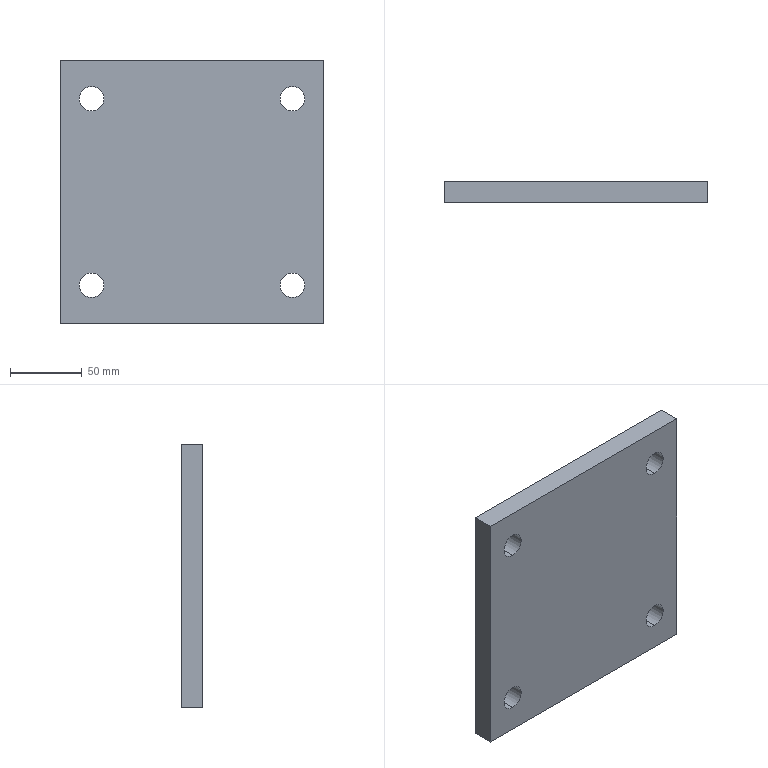Part | SolidWorks | features BaseBody 1 | 1 solid | 14 faces | box 184 x 15 x 184 mm | volume 494221 mm3 | cylinder 8 | plane 6 | commonest cylinder face diameters 17 x8
STEP:
#1=CARTESIAN_POINT('',(70.,64.2,-76.379));
#2=VERTEX_POINT('',#1);
#3=CARTESIAN_POINT('',(70.,64.2,-93.379));
#4=VERTEX_POINT('',#3);
#5=CARTESIAN_POINT('',(70.,64.2,-84.879));
#6=DIRECTION('',(0.,-1.,0.));
#7=DIRECTION('',(0.,0.,-1.));
#8=AXIS2_PLACEMENT_3D('',#5,#6,#7);
#9=CIRCLE('',#8,8.5);
#10=EDGE_CURVE('',#2,#4,#9,.T.);
#11=ORIENTED_EDGE('',*,*,#10,.F.);
#12=CARTESIAN_POINT('',(70.,49.2,-76.379));
#13=VERTEX_POINT('',#12);
#14=CARTESIAN_POINT('',(70.,64.201,-76.379));
#15=DIRECTION('',(0.,-1.,0.));
#16=VECTOR('',#15,1000.);
#17=LINE('',#14,#16);
#18=EDGE_CURVE('',#2,#13,#17,.T.);
#19=ORIENTED_EDGE('',*,*,#18,.T.);
#20=CARTESIAN_POINT('',(70.,49.2,-93.379));
#21=VERTEX_POINT('',#20);
#22=CARTESIAN_POINT('',(70.,49.2,-84.879));
#23=DIRECTION('',(0.,-1.,0.));
#24=DIRECTION('',(0.,0.,-1.));
#25=AXIS2_PLACEMENT_3D('',#22,#23,#24);
#26=CIRCLE('',#25,8.5);
#27=EDGE_CURVE('',#13,#21,#26,.T.);
#28=ORIENTED_EDGE('',*,*,#27,.T.);
#29=CARTESIAN_POINT('',(70.,64.201,-93.379));
#30=DIRECTION('',(0.,-1.,0.));
#31=VECTOR('',#30,1000.);
#32=LINE('',#29,#31);
#33=EDGE_CURVE('',#4,#21,#32,.T.);
#34=ORIENTED_EDGE('',*,*,#33,.F.);
#35=EDGE_LOOP('',(#11,#19,#28,#34));
#36=FACE_OUTER_BOUND('',#35,.T.);
#37=CARTESIAN_POINT('',(70.,64.201,-84.879));
#38=DIRECTION('',(0.,-1.,0.));
#39=DIRECTION('',(0.,0.,-1.));
#40=AXIS2_PLACEMENT_3D('',#37,#38,#39);
#41=CYLINDRICAL_SURFACE('',#40,8.5);
#42=ADVANCED_FACE('',(#36),#41,.F.);
#43=CARTESIAN_POINT('',(70.,64.2,-206.379));
#44=VERTEX_POINT('',#43);
#45=CARTESIAN_POINT('',(70.,64.2,-223.379));
#46=VERTEX_POINT('',#45);
#47=CARTESIAN_POINT('',(70.,64.2,-214.879));
#48=DIRECTION('',(0.,-1.,0.));
#49=DIRECTION('',(0.,0.,-1.));
#50=AXIS2_PLACEMENT_3D('',#47,#48,#49);
#51=CIRCLE('',#50,8.5);
#52=EDGE_CURVE('',#44,#46,#51,.T.);
#53=ORIENTED_EDGE('',*,*,#52,.F.);
#54=CARTESIAN_POINT('',(70.,49.2,-206.379));
#55=VERTEX_POINT('',#54);
#56=CARTESIAN_POINT('',(70.,64.201,-206.379));
#57=DIRECTION('',(0.,-1.,0.));
#58=VECTOR('',#57,1000.);
#59=LINE('',#56,#58);
#60=EDGE_CURVE('',#44,#55,#59,.T.);
#61=ORIENTED_EDGE('',*,*,#60,.T.);
#62=CARTESIAN_POINT('',(70.,49.2,-223.379));
#63=VERTEX_POINT('',#62);
#64=CARTESIAN_POINT('',(70.,49.2,-214.879));
#65=DIRECTION('',(0.,-1.,0.));
#66=DIRECTION('',(0.,0.,-1.));
#67=AXIS2_PLACEMENT_3D('',#64,#65,#66);
#68=CIRCLE('',#67,8.5);
#69=EDGE_CURVE('',#55,#63,#68,.T.);
#70=ORIENTED_EDGE('',*,*,#69,.T.);
#71=CARTESIAN_POINT('',(70.,64.201,-223.379));
#72=DIRECTION('',(0.,-1.,0.));
#73=VECTOR('',#72,1000.);
#74=LINE('',#71,#73);
#75=EDGE_CURVE('',#46,#63,#74,.T.);
#76=ORIENTED_EDGE('',*,*,#75,.F.);
#77=EDGE_LOOP('',(#53,#61,#70,#76));
#78=FACE_OUTER_BOUND('',#77,.T.);
#79=CARTESIAN_POINT('',(70.,64.201,-214.879));
#80=DIRECTION('',(0.,-1.,0.));
#81=DIRECTION('',(0.,0.,-1.));
#82=AXIS2_PLACEMENT_3D('',#79,#80,#81);
#83=CYLINDRICAL_SURFACE('',#82,8.5);
#84=ADVANCED_FACE('',(#78),#83,.F.);
#85=CARTESIAN_POINT('',(-70.,64.2,-76.379));
#86=VERTEX_POINT('',#85);
#87=CARTESIAN_POINT('',(-70.,64.2,-93.379));
#88=VERTEX_POINT('',#87);
#89=CARTESIAN_POINT('',(-70.,64.2,-84.879));
#90=DIRECTION('',(0.,-1.,0.));
#91=DIRECTION('',(0.,0.,-1.));
#92=AXIS2_PLACEMENT_3D('',#89,#90,#91);
#93=CIRCLE('',#92,8.5);
#94=EDGE_CURVE('',#86,#88,#93,.T.);
#95=ORIENTED_EDGE('',*,*,#94,.F.);
#96=CARTESIAN_POINT('',(-70.,49.2,-76.379));
#97=VERTEX_POINT('',#96);
#98=CARTESIAN_POINT('',(-70.,64.201,-76.379));
#99=DIRECTION('',(0.,-1.,0.));
#100=VECTOR('',#99,1000.);
#101=LINE('',#98,#100);
#102=EDGE_CURVE('',#86,#97,#101,.T.);
#103=ORIENTED_EDGE('',*,*,#102,.T.);
#104=CARTESIAN_POINT('',(-70.,49.2,-93.379));
#105=VERTEX_POINT('',#104);
#106=CARTESIAN_POINT('',(-70.,49.2,-84.879));
#107=DIRECTION('',(0.,-1.,0.));
#108=DIRECTION('',(0.,0.,-1.));
#109=AXIS2_PLACEMENT_3D('',#106,#107,#108);
#110=CIRCLE('',#109,8.5);
#111=EDGE_CURVE('',#97,#105,#110,.T.);
#112=ORIENTED_EDGE('',*,*,#111,.T.);
#113=CARTESIAN_POINT('',(-70.,64.201,-93.379));
#114=DIRECTION('',(0.,-1.,0.));
#115=VECTOR('',#114,1000.);
#116=LINE('',#113,#115);
#117=EDGE_CURVE('',#88,#105,#116,.T.);
#118=ORIENTED_EDGE('',*,*,#117,.F.);
#119=EDGE_LOOP('',(#95,#103,#112,#118));
#120=FACE_OUTER_BOUND('',#119,.T.);
#121=CARTESIAN_POINT('',(-70.,64.201,-84.879));
#122=DIRECTION('',(0.,-1.,0.));
#123=DIRECTION('',(0.,0.,-1.));
#124=AXIS2_PLACEMENT_3D('',#121,#122,#123);
#125=CYLINDRICAL_SURFACE('',#124,8.5);
#126=ADVANCED_FACE('',(#120),#125,.F.);
#127=CARTESIAN_POINT('',(-70.,64.2,-206.379));
#128=VERTEX_POINT('',#127);
#129=CARTESIAN_POINT('',(-70.,64.2,-223.379));
#130=VERTEX_POINT('',#129);
#131=CARTESIAN_POINT('',(-70.,64.2,-214.879));
#132=DIRECTION('',(0.,-1.,0.));
#133=DIRECTION('',(0.,0.,-1.));
#134=AXIS2_PLACEMENT_3D('',#131,#132,#133);
#135=CIRCLE('',#134,8.5);
#136=EDGE_CURVE('',#128,#130,#135,.T.);
#137=ORIENTED_EDGE('',*,*,#136,.F.);
#138=CARTESIAN_POINT('',(-70.,49.2,-206.379));
#139=VERTEX_POINT('',#138);
#140=CARTESIAN_POINT('',(-70.,64.201,-206.379));
#141=DIRECTION('',(0.,-1.,0.));
#142=VECTOR('',#141,1000.);
#143=LINE('',#140,#142);
#144=EDGE_CURVE('',#128,#139,#143,.T.);
#145=ORIENTED_EDGE('',*,*,#144,.T.);
#146=CARTESIAN_POINT('',(-70.,49.2,-223.379));
#147=VERTEX_POINT('',#146);
#148=CARTESIAN_POINT('',(-70.,49.2,-214.879));
#149=DIRECTION('',(0.,-1.,0.));
#150=DIRECTION('',(0.,0.,-1.));
#151=AXIS2_PLACEMENT_3D('',#148,#149,#150);
#152=CIRCLE('',#151,8.5);
#153=EDGE_CURVE('',#139,#147,#152,.T.);
#154=ORIENTED_EDGE('',*,*,#153,.T.);
#155=CARTESIAN_POINT('',(-70.,64.201,-223.379));
#156=DIRECTION('',(0.,-1.,0.));
#157=VECTOR('',#156,1000.);
#158=LINE('',#155,#157);
#159=EDGE_CURVE('',#130,#147,#158,.T.);
#160=ORIENTED_EDGE('',*,*,#159,.F.);
#161=EDGE_LOOP('',(#137,#145,#154,#160));
#162=FACE_OUTER_BOUND('',#161,.T.);
#163=CARTESIAN_POINT('',(-70.,64.201,-214.879));
#164=DIRECTION('',(0.,-1.,0.));
#165=DIRECTION('',(0.,0.,-1.));
#166=AXIS2_PLACEMENT_3D('',#163,#164,#165);
#167=CYLINDRICAL_SURFACE('',#166,8.5);
#168=ADVANCED_FACE('',(#162),#167,.F.);
#169=CARTESIAN_POINT('',(-92.,49.2,-57.879));
#170=VERTEX_POINT('',#169);
#171=CARTESIAN_POINT('',(92.,49.2,-57.879));
#172=VERTEX_POINT('',#171);
#173=CARTESIAN_POINT('',(0.,49.2,-57.879));
#174=DIRECTION('',(1.,0.,0.));
#175=VECTOR('',#174,1000.);
#176=LINE('',#173,#175);
#177=EDGE_CURVE('',#170,#172,#176,.T.);
#178=ORIENTED_EDGE('',*,*,#177,.F.);
#179=CARTESIAN_POINT('',(-92.,49.2,-241.879));
#180=VERTEX_POINT('',#179);
#181=CARTESIAN_POINT('',(-92.,49.2,-149.879));
#182=DIRECTION('',(0.,0.,1.));
#183=VECTOR('',#182,1000.);
#184=LINE('',#181,#183);
#185=EDGE_CURVE('',#180,#170,#184,.T.);
#186=ORIENTED_EDGE('',*,*,#185,.F.);
#187=CARTESIAN_POINT('',(92.,49.2,-241.879));
#188=VERTEX_POINT('',#187);
#189=CARTESIAN_POINT('',(0.,49.2,-241.879));
#190=DIRECTION('',(-1.,0.,0.));
#191=VECTOR('',#190,1000.);
#192=LINE('',#189,#191);
#193=EDGE_CURVE('',#188,#180,#192,.T.);
#194=ORIENTED_EDGE('',*,*,#193,.F.);
#195=CARTESIAN_POINT('',(92.,49.2,-149.879));
#196=DIRECTION('',(0.,0.,-1.));
#197=VECTOR('',#196,1000.);
#198=LINE('',#195,#197);
#199=EDGE_CURVE('',#172,#188,#198,.T.);
#200=ORIENTED_EDGE('',*,*,#199,.F.);
#201=EDGE_LOOP('',(#178,#186,#194,#200));
#202=FACE_OUTER_BOUND('',#201,.T.);
#203=CARTESIAN_POINT('',(70.,49.2,-84.879));
#204=DIRECTION('',(0.,-1.,0.));
#205=DIRECTION('',(0.,0.,-1.));
#206=AXIS2_PLACEMENT_3D('',#203,#204,#205);
#207=CIRCLE('',#206,8.5);
#208=EDGE_CURVE('',#21,#13,#207,.T.);
#209=ORIENTED_EDGE('',*,*,#208,.F.);
#210=ORIENTED_EDGE('',*,*,#27,.F.);
#211=EDGE_LOOP('',(#209,#210));
#212=FACE_BOUND('',#211,.T.);
#213=CARTESIAN_POINT('',(70.,49.2,-214.879));
#214=DIRECTION('',(0.,-1.,0.));
#215=DIRECTION('',(0.,0.,-1.));
#216=AXIS2_PLACEMENT_3D('',#213,#214,#215);
#217=CIRCLE('',#216,8.5);
#218=EDGE_CURVE('',#63,#55,#217,.T.);
#219=ORIENTED_EDGE('',*,*,#218,.F.);
#220=ORIENTED_EDGE('',*,*,#69,.F.);
#221=EDGE_LOOP('',(#219,#220));
#222=FACE_BOUND('',#221,.T.);
#223=CARTESIAN_POINT('',(-70.,49.2,-84.879));
#224=DIRECTION('',(0.,-1.,0.));
#225=DIRECTION('',(0.,0.,-1.));
#226=AXIS2_PLACEMENT_3D('',#223,#224,#225);
#227=CIRCLE('',#226,8.5);
#228=EDGE_CURVE('',#105,#97,#227,.T.);
#229=ORIENTED_EDGE('',*,*,#228,.F.);
#230=ORIENTED_EDGE('',*,*,#111,.F.);
#231=EDGE_LOOP('',(#229,#230));
#232=FACE_BOUND('',#231,.T.);
#233=CARTESIAN_POINT('',(-70.,49.2,-214.879));
#234=DIRECTION('',(0.,-1.,0.));
#235=DIRECTION('',(0.,0.,-1.));
#236=AXIS2_PLACEMENT_3D('',#233,#234,#235);
#237=CIRCLE('',#236,8.5);
#238=EDGE_CURVE('',#147,#139,#237,.T.);
#239=ORIENTED_EDGE('',*,*,#238,.F.);
#240=ORIENTED_EDGE('',*,*,#153,.F.);
#241=EDGE_LOOP('',(#239,#240));
#242=FACE_BOUND('',#241,.T.);
#243=CARTESIAN_POINT('',(0.,49.2,-149.879));
#244=DIRECTION('',(0.,1.,0.));
#245=DIRECTION('',(0.,0.,1.));
#246=AXIS2_PLACEMENT_3D('',#243,#244,#245);
#247=PLANE('',#246);
#248=ADVANCED_FACE('',(#202,#212,#222,#232,#242),#247,.F.);
#249=CARTESIAN_POINT('',(92.,64.2,-57.879));
#250=VERTEX_POINT('',#249);
#251=CARTESIAN_POINT('',(92.,49.2,-57.879));
#252=DIRECTION('',(0.,1.,0.));
#253=VECTOR('',#252,1000.);
#254=LINE('',#251,#253);
#255=EDGE_CURVE('',#172,#250,#254,.T.);
#256=ORIENTED_EDGE('',*,*,#255,.F.);
#257=ORIENTED_EDGE('',*,*,#199,.T.);
#258=CARTESIAN_POINT('',(92.,64.2,-241.879));
#259=VERTEX_POINT('',#258);
#260=CARTESIAN_POINT('',(92.,49.2,-241.879));
#261=DIRECTION('',(0.,-1.,0.));
#262=VECTOR('',#261,1000.);
#263=LINE('',#260,#262);
#264=EDGE_CURVE('',#259,#188,#263,.T.);
#265=ORIENTED_EDGE('',*,*,#264,.F.);
#266=CARTESIAN_POINT('',(92.,64.2,-241.879));
#267=DIRECTION('',(0.,0.,-1.));
#268=VECTOR('',#267,1000.);
#269=LINE('',#266,#268);
#270=EDGE_CURVE('',#250,#259,#269,.T.);
#271=ORIENTED_EDGE('',*,*,#270,.F.);
#272=EDGE_LOOP('',(#256,#257,#265,#271));
#273=FACE_OUTER_BOUND('',#272,.T.);
#274=CARTESIAN_POINT('',(92.,49.2,-241.879));
#275=DIRECTION('',(-1.,0.,0.));
#276=DIRECTION('',(0.,0.,1.));
#277=AXIS2_PLACEMENT_3D('',#274,#275,#276);
#278=PLANE('',#277);
#279=ADVANCED_FACE('',(#273),#278,.F.);
#280=CARTESIAN_POINT('',(-92.,64.2,-57.879));
#281=VERTEX_POINT('',#280);
#282=CARTESIAN_POINT('',(-92.,49.2,-57.879));
#283=DIRECTION('',(0.,1.,0.));
#284=VECTOR('',#283,1000.);
#285=LINE('',#282,#284);
#286=EDGE_CURVE('',#170,#281,#285,.T.);
#287=ORIENTED_EDGE('',*,*,#286,.F.);
#288=ORIENTED_EDGE('',*,*,#177,.T.);
#289=ORIENTED_EDGE('',*,*,#255,.T.);
#290=CARTESIAN_POINT('',(-92.,64.2,-57.879));
#291=DIRECTION('',(1.,0.,0.));
#292=VECTOR('',#291,1000.);
#293=LINE('',#290,#292);
#294=EDGE_CURVE('',#281,#250,#293,.T.);
#295=ORIENTED_EDGE('',*,*,#294,.F.);
#296=EDGE_LOOP('',(#287,#288,#289,#295));
#297=FACE_OUTER_BOUND('',#296,.T.);
#298=CARTESIAN_POINT('',(-92.,49.2,-57.879));
#299=DIRECTION('',(0.,0.,-1.));
#300=DIRECTION('',(-1.,0.,0.));
#301=AXIS2_PLACEMENT_3D('',#298,#299,#300);
#302=PLANE('',#301);
#303=ADVANCED_FACE('',(#297),#302,.F.);
#304=CARTESIAN_POINT('',(-92.,64.2,-241.879));
#305=VERTEX_POINT('',#304);
#306=CARTESIAN_POINT('',(-92.,49.2,-241.879));
#307=DIRECTION('',(0.,1.,0.));
#308=VECTOR('',#307,1000.);
#309=LINE('',#306,#308);
#310=EDGE_CURVE('',#180,#305,#309,.T.);
#311=ORIENTED_EDGE('',*,*,#310,.F.);
#312=ORIENTED_EDGE('',*,*,#185,.T.);
#313=ORIENTED_EDGE('',*,*,#286,.T.);
#314=CARTESIAN_POINT('',(-92.,64.2,-241.879));
#315=DIRECTION('',(0.,0.,1.));
#316=VECTOR('',#315,1000.);
#317=LINE('',#314,#316);
#318=EDGE_CURVE('',#305,#281,#317,.T.);
#319=ORIENTED_EDGE('',*,*,#318,.F.);
#320=EDGE_LOOP('',(#311,#312,#313,#319));
#321=FACE_OUTER_BOUND('',#320,.T.);
#322=CARTESIAN_POINT('',(-92.,49.2,-241.879));
#323=DIRECTION('',(1.,0.,0.));
#324=DIRECTION('',(0.,0.,-1.));
#325=AXIS2_PLACEMENT_3D('',#322,#323,#324);
#326=PLANE('',#325);
#327=ADVANCED_FACE('',(#321),#326,.F.);
#328=ORIENTED_EDGE('',*,*,#264,.T.);
#329=ORIENTED_EDGE('',*,*,#193,.T.);
#330=ORIENTED_EDGE('',*,*,#310,.T.);
#331=CARTESIAN_POINT('',(-92.,64.2,-241.879));
#332=DIRECTION('',(-1.,0.,0.));
#333=VECTOR('',#332,1000.);
#334=LINE('',#331,#333);
#335=EDGE_CURVE('',#259,#305,#334,.T.);
#336=ORIENTED_EDGE('',*,*,#335,.F.);
#337=EDGE_LOOP('',(#328,#329,#330,#336));
#338=FACE_OUTER_BOUND('',#337,.T.);
#339=CARTESIAN_POINT('',(-92.,49.2,-241.879));
#340=DIRECTION('',(0.,0.,1.));
#341=DIRECTION('',(1.,0.,0.));
#342=AXIS2_PLACEMENT_3D('',#339,#340,#341);
#343=PLANE('',#342);
#344=ADVANCED_FACE('',(#338),#343,.F.);
#345=ORIENTED_EDGE('',*,*,#18,.F.);
#346=CARTESIAN_POINT('',(70.,64.2,-84.879));
#347=DIRECTION('',(0.,-1.,0.));
#348=DIRECTION('',(0.,0.,-1.));
#349=AXIS2_PLACEMENT_3D('',#346,#347,#348);
#350=CIRCLE('',#349,8.5);
#351=EDGE_CURVE('',#4,#2,#350,.T.);
#352=ORIENTED_EDGE('',*,*,#351,.F.);
#353=ORIENTED_EDGE('',*,*,#33,.T.);
#354=ORIENTED_EDGE('',*,*,#208,.T.);
#355=EDGE_LOOP('',(#345,#352,#353,#354));
#356=FACE_OUTER_BOUND('',#355,.T.);
#357=CARTESIAN_POINT('',(70.,64.201,-84.879));
#358=DIRECTION('',(0.,-1.,0.));
#359=DIRECTION('',(0.,0.,-1.));
#360=AXIS2_PLACEMENT_3D('',#357,#358,#359);
#361=CYLINDRICAL_SURFACE('',#360,8.5);
#362=ADVANCED_FACE('',(#356),#361,.F.);
#363=ORIENTED_EDGE('',*,*,#60,.F.);
#364=CARTESIAN_POINT('',(70.,64.2,-214.879));
#365=DIRECTION('',(0.,-1.,0.));
#366=DIRECTION('',(0.,0.,-1.));
#367=AXIS2_PLACEMENT_3D('',#364,#365,#366);
#368=CIRCLE('',#367,8.5);
#369=EDGE_CURVE('',#46,#44,#368,.T.);
#370=ORIENTED_EDGE('',*,*,#369,.F.);
#371=ORIENTED_EDGE('',*,*,#75,.T.);
#372=ORIENTED_EDGE('',*,*,#218,.T.);
#373=EDGE_LOOP('',(#363,#370,#371,#372));
#374=FACE_OUTER_BOUND('',#373,.T.);
#375=CARTESIAN_POINT('',(70.,64.201,-214.879));
#376=DIRECTION('',(0.,-1.,0.));
#377=DIRECTION('',(0.,0.,-1.));
#378=AXIS2_PLACEMENT_3D('',#375,#376,#377);
#379=CYLINDRICAL_SURFACE('',#378,8.5);
#380=ADVANCED_FACE('',(#374),#379,.F.);
#381=ORIENTED_EDGE('',*,*,#102,.F.);
#382=CARTESIAN_POINT('',(-70.,64.2,-84.879));
#383=DIRECTION('',(0.,-1.,0.));
#384=DIRECTION('',(0.,0.,-1.));
#385=AXIS2_PLACEMENT_3D('',#382,#383,#384);
#386=CIRCLE('',#385,8.5);
#387=EDGE_CURVE('',#88,#86,#386,.T.);
#388=ORIENTED_EDGE('',*,*,#387,.F.);
#389=ORIENTED_EDGE('',*,*,#117,.T.);
#390=ORIENTED_EDGE('',*,*,#228,.T.);
#391=EDGE_LOOP('',(#381,#388,#389,#390));
#392=FACE_OUTER_BOUND('',#391,.T.);
#393=CARTESIAN_POINT('',(-70.,64.201,-84.879));
#394=DIRECTION('',(0.,-1.,0.));
#395=DIRECTION('',(0.,0.,-1.));
#396=AXIS2_PLACEMENT_3D('',#393,#394,#395);
#397=CYLINDRICAL_SURFACE('',#396,8.5);
#398=ADVANCED_FACE('',(#392),#397,.F.);
#399=ORIENTED_EDGE('',*,*,#144,.F.);
#400=CARTESIAN_POINT('',(-70.,64.2,-214.879));
#401=DIRECTION('',(0.,-1.,0.));
#402=DIRECTION('',(0.,0.,-1.));
#403=AXIS2_PLACEMENT_3D('',#400,#401,#402);
#404=CIRCLE('',#403,8.5);
#405=EDGE_CURVE('',#130,#128,#404,.T.);
#406=ORIENTED_EDGE('',*,*,#405,.F.);
#407=ORIENTED_EDGE('',*,*,#159,.T.);
#408=ORIENTED_EDGE('',*,*,#238,.T.);
#409=EDGE_LOOP('',(#399,#406,#407,#408));
#410=FACE_OUTER_BOUND('',#409,.T.);
#411=CARTESIAN_POINT('',(-70.,64.201,-214.879));
#412=DIRECTION('',(0.,-1.,0.));
#413=DIRECTION('',(0.,0.,-1.));
#414=AXIS2_PLACEMENT_3D('',#411,#412,#413);
#415=CYLINDRICAL_SURFACE('',#414,8.5);
#416=ADVANCED_FACE('',(#410),#415,.F.);
#417=ORIENTED_EDGE('',*,*,#318,.T.);
#418=ORIENTED_EDGE('',*,*,#294,.T.);
#419=ORIENTED_EDGE('',*,*,#270,.T.);
#420=ORIENTED_EDGE('',*,*,#335,.T.);
#421=EDGE_LOOP('',(#417,#418,#419,#420));
#422=FACE_OUTER_BOUND('',#421,.T.);
#423=ORIENTED_EDGE('',*,*,#351,.T.);
#424=ORIENTED_EDGE('',*,*,#10,.T.);
#425=EDGE_LOOP('',(#423,#424));
#426=FACE_BOUND('',#425,.T.);
#427=ORIENTED_EDGE('',*,*,#369,.T.);
#428=ORIENTED_EDGE('',*,*,#52,.T.);
#429=EDGE_LOOP('',(#427,#428));
#430=FACE_BOUND('',#429,.T.);
#431=ORIENTED_EDGE('',*,*,#387,.T.);
#432=ORIENTED_EDGE('',*,*,#94,.T.);
#433=EDGE_LOOP('',(#431,#432));
#434=FACE_BOUND('',#433,.T.);
#435=ORIENTED_EDGE('',*,*,#405,.T.);
#436=ORIENTED_EDGE('',*,*,#136,.T.);
#437=EDGE_LOOP('',(#435,#436));
#438=FACE_BOUND('',#437,.T.);
#439=CARTESIAN_POINT('',(0.,64.2,-149.879));
#440=DIRECTION('',(0.,1.,0.));
#441=DIRECTION('',(0.,0.,1.));
#442=AXIS2_PLACEMENT_3D('',#439,#440,#441);
#443=PLANE('',#442);
#444=ADVANCED_FACE('',(#422,#426,#430,#434,#438),#443,.T.);
#445=CLOSED_SHELL('',(#42,#84,#126,#168,#248,#279,#303,#327,#344,#362,#380,#398,#416,#444));
#446=MANIFOLD_SOLID_BREP('',#445);
#447=CARTESIAN_POINT('',(0.,0.,0.));
#448=DIRECTION('',(0.,0.,1.));
#449=DIRECTION('',(1.,0.,0.));
#450=AXIS2_PLACEMENT_3D('',#447,#448,#449);
#451=(LENGTH_UNIT()NAMED_UNIT(*)SI_UNIT(.MILLI.,.METRE.));
#452=UNCERTAINTY_MEASURE_WITH_UNIT(LENGTH_MEASURE(0.00001),#451,'','');
#453=(NAMED_UNIT(*)PLANE_ANGLE_UNIT()SI_UNIT($,.RADIAN.));
#454=(NAMED_UNIT(*)SI_UNIT($,.STERADIAN.)SOLID_ANGLE_UNIT());
#455=(GEOMETRIC_REPRESENTATION_CONTEXT(3)GLOBAL_UNCERTAINTY_ASSIGNED_CONTEXT((#452))GLOBAL_UNIT_ASSIGNED_CONTEXT((#451,#453,#454))REPRESENTATION_CONTEXT('',''));
#456=ADVANCED_BREP_SHAPE_REPRESENTATION('',(#446,#450),#455);